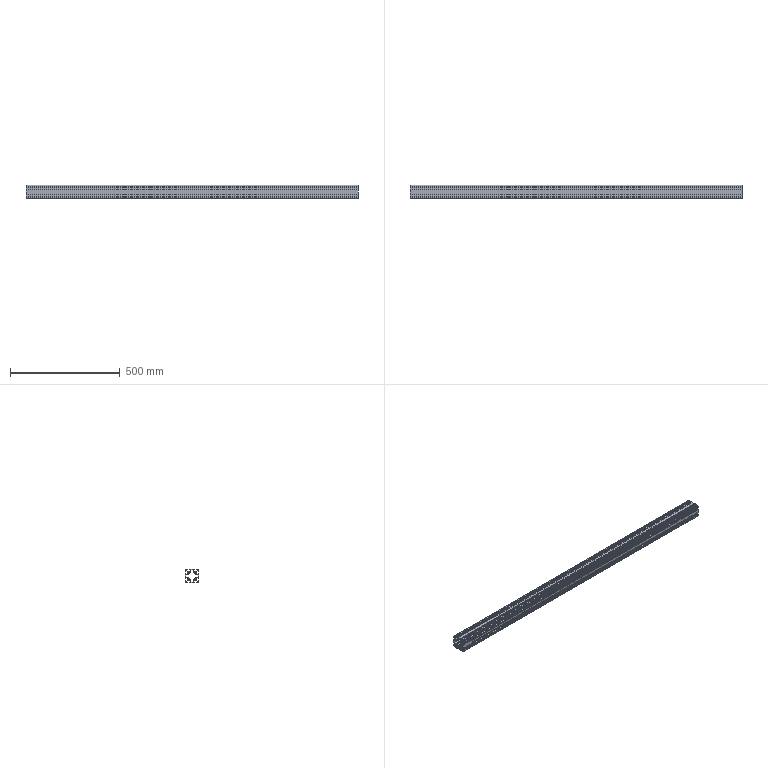Part | STEP file | PN_0019 Square aluminium tube_Default <Machined> | 1 solid | 178 faces | box 1510 x 60 x 60 mm | volume 1389788 mm3 | plane 162 | cylinder 16 | commonest cylinder face diameters 6.8 x8 6.76 x4 11.828 x4